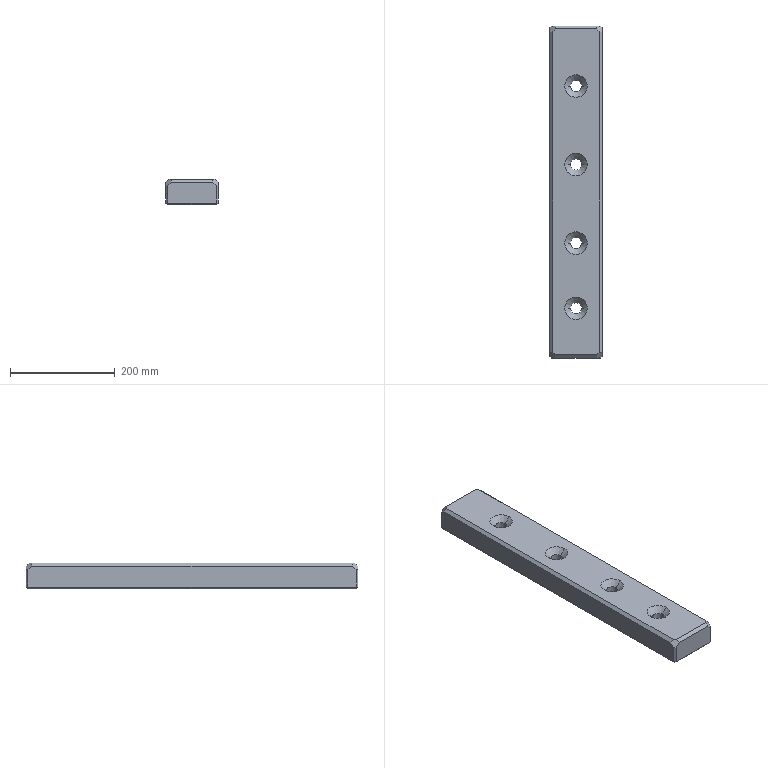Part | Creo | 1 solid | 50 faces | box 100 x 635 x 49.3 mm | volume 3002478 mm3 | plane 26 | cone 16 | cylinder 8 | commonest cylinder face diameters 21.5 x8
STEP:
#1=CARTESIAN_POINT('',(0.,0.,0.));
#2=DIRECTION('',(0.,0.,1.));
#3=DIRECTION('',(1.,0.,0.));
#4=AXIS2_PLACEMENT_3D('',#1,#2,#3);
#5=CARTESIAN_POINT('',(473.372,294.801,305.059));
#6=VERTEX_POINT('',#5);
#7=CARTESIAN_POINT('',(473.372,-319.056,305.059));
#8=VERTEX_POINT('',#7);
#9=CARTESIAN_POINT('',(473.372,294.801,305.059));
#10=DIRECTION('',(0.,-1.,0.));
#11=VECTOR('',#10,613.858);
#12=LINE('',#9,#11);
#13=EDGE_CURVE('',#6,#8,#12,.T.);
#14=ORIENTED_EDGE('',*,*,#13,.T.);
#15=CARTESIAN_POINT('',(468.53,-323.899,305.059));
#16=VERTEX_POINT('',#15);
#17=CARTESIAN_POINT('',(473.372,-319.056,305.059));
#18=DIRECTION('',(-0.7071,-0.7071,0.));
#19=VECTOR('',#18,6.848);
#20=LINE('',#17,#19);
#21=EDGE_CURVE('',#8,#16,#20,.T.);
#22=ORIENTED_EDGE('',*,*,#21,.T.);
#23=CARTESIAN_POINT('',(389.672,-323.899,305.059));
#24=VERTEX_POINT('',#23);
#25=CARTESIAN_POINT('',(468.53,-323.899,305.059));
#26=DIRECTION('',(-1.,0.,0.));
#27=VECTOR('',#26,78.858);
#28=LINE('',#25,#27);
#29=EDGE_CURVE('',#16,#24,#28,.T.);
#30=ORIENTED_EDGE('',*,*,#29,.T.);
#31=CARTESIAN_POINT('',(384.83,-319.056,305.059));
#32=VERTEX_POINT('',#31);
#33=CARTESIAN_POINT('',(389.672,-323.899,305.059));
#34=DIRECTION('',(-0.7071,0.7071,0.));
#35=VECTOR('',#34,6.848);
#36=LINE('',#33,#35);
#37=EDGE_CURVE('',#24,#32,#36,.T.);
#38=ORIENTED_EDGE('',*,*,#37,.T.);
#39=CARTESIAN_POINT('',(384.83,294.801,305.059));
#40=VERTEX_POINT('',#39);
#41=CARTESIAN_POINT('',(384.83,-319.056,305.059));
#42=DIRECTION('',(0.,1.,0.));
#43=VECTOR('',#42,613.858);
#44=LINE('',#41,#43);
#45=EDGE_CURVE('',#32,#40,#44,.T.);
#46=ORIENTED_EDGE('',*,*,#45,.T.);
#47=CARTESIAN_POINT('',(389.672,299.644,305.059));
#48=VERTEX_POINT('',#47);
#49=CARTESIAN_POINT('',(389.672,299.644,305.059));
#50=DIRECTION('',(-0.7071,-0.7071,0.));
#51=VECTOR('',#50,6.848);
#52=LINE('',#49,#51);
#53=EDGE_CURVE('',#48,#40,#52,.T.);
#54=ORIENTED_EDGE('',*,*,#53,.F.);
#55=CARTESIAN_POINT('',(468.53,299.644,305.059));
#56=VERTEX_POINT('',#55);
#57=CARTESIAN_POINT('',(389.672,299.644,305.059));
#58=DIRECTION('',(1.,0.,0.));
#59=VECTOR('',#58,78.858);
#60=LINE('',#57,#59);
#61=EDGE_CURVE('',#48,#56,#60,.T.);
#62=ORIENTED_EDGE('',*,*,#61,.T.);
#63=CARTESIAN_POINT('',(468.53,299.644,305.059));
#64=DIRECTION('',(0.7071,-0.7071,0.));
#65=VECTOR('',#64,6.848);
#66=LINE('',#63,#65);
#67=EDGE_CURVE('',#56,#6,#66,.T.);
#68=ORIENTED_EDGE('',*,*,#67,.T.);
#69=EDGE_LOOP('',(#14,#22,#30,#38,#46,#54,#62,#68));
#70=FACE_OUTER_BOUND('',#69,.F.);
#71=CARTESIAN_POINT('',(450.651,-234.627,305.059));
#72=VERTEX_POINT('',#71);
#73=CARTESIAN_POINT('',(407.551,-234.627,305.059));
#74=VERTEX_POINT('',#73);
#75=CARTESIAN_POINT('',(429.101,-234.627,305.059));
#76=DIRECTION('',(0.,0.,-1.));
#77=DIRECTION('',(1.,0.,0.));
#78=AXIS2_PLACEMENT_3D('',#75,#76,#77);
#79=CIRCLE('',#78,21.55);
#80=EDGE_CURVE('',#72,#74,#79,.T.);
#81=ORIENTED_EDGE('',*,*,#80,.F.);
#82=CARTESIAN_POINT('',(429.101,-234.627,305.059));
#83=DIRECTION('',(0.,0.,-1.));
#84=DIRECTION('',(-1.,0.,0.));
#85=AXIS2_PLACEMENT_3D('',#82,#83,#84);
#86=CIRCLE('',#85,21.55);
#87=EDGE_CURVE('',#74,#72,#86,.T.);
#88=ORIENTED_EDGE('',*,*,#87,.F.);
#89=EDGE_LOOP('',(#81,#88));
#90=FACE_BOUND('',#89,.F.);
#91=CARTESIAN_POINT('',(450.651,-110.,305.059));
#92=VERTEX_POINT('',#91);
#93=CARTESIAN_POINT('',(407.551,-110.,305.059));
#94=VERTEX_POINT('',#93);
#95=CARTESIAN_POINT('',(429.101,-110.,305.059));
#96=DIRECTION('',(0.,0.,-1.));
#97=DIRECTION('',(1.,0.,0.));
#98=AXIS2_PLACEMENT_3D('',#95,#96,#97);
#99=CIRCLE('',#98,21.55);
#100=EDGE_CURVE('',#92,#94,#99,.T.);
#101=ORIENTED_EDGE('',*,*,#100,.F.);
#102=CARTESIAN_POINT('',(429.101,-110.,305.059));
#103=DIRECTION('',(0.,0.,-1.));
#104=DIRECTION('',(-1.,0.,0.));
#105=AXIS2_PLACEMENT_3D('',#102,#103,#104);
#106=CIRCLE('',#105,21.55);
#107=EDGE_CURVE('',#94,#92,#106,.T.);
#108=ORIENTED_EDGE('',*,*,#107,.F.);
#109=EDGE_LOOP('',(#101,#108));
#110=FACE_BOUND('',#109,.F.);
#111=CARTESIAN_POINT('',(450.651,40.373,305.059));
#112=VERTEX_POINT('',#111);
#113=CARTESIAN_POINT('',(407.551,40.373,305.059));
#114=VERTEX_POINT('',#113);
#115=CARTESIAN_POINT('',(429.101,40.373,305.059));
#116=DIRECTION('',(0.,0.,-1.));
#117=DIRECTION('',(1.,0.,0.));
#118=AXIS2_PLACEMENT_3D('',#115,#116,#117);
#119=CIRCLE('',#118,21.55);
#120=EDGE_CURVE('',#112,#114,#119,.T.);
#121=ORIENTED_EDGE('',*,*,#120,.F.);
#122=CARTESIAN_POINT('',(429.101,40.373,305.059));
#123=DIRECTION('',(0.,0.,-1.));
#124=DIRECTION('',(-1.,0.,0.));
#125=AXIS2_PLACEMENT_3D('',#122,#123,#124);
#126=CIRCLE('',#125,21.55);
#127=EDGE_CURVE('',#114,#112,#126,.T.);
#128=ORIENTED_EDGE('',*,*,#127,.F.);
#129=EDGE_LOOP('',(#121,#128));
#130=FACE_BOUND('',#129,.F.);
#131=CARTESIAN_POINT('',(450.651,190.373,305.059));
#132=VERTEX_POINT('',#131);
#133=CARTESIAN_POINT('',(407.551,190.373,305.059));
#134=VERTEX_POINT('',#133);
#135=CARTESIAN_POINT('',(429.101,190.373,305.059));
#136=DIRECTION('',(0.,0.,-1.));
#137=DIRECTION('',(1.,0.,0.));
#138=AXIS2_PLACEMENT_3D('',#135,#136,#137);
#139=CIRCLE('',#138,21.55);
#140=EDGE_CURVE('',#132,#134,#139,.T.);
#141=ORIENTED_EDGE('',*,*,#140,.F.);
#142=CARTESIAN_POINT('',(429.101,190.373,305.059));
#143=DIRECTION('',(0.,0.,-1.));
#144=DIRECTION('',(-1.,0.,0.));
#145=AXIS2_PLACEMENT_3D('',#142,#143,#144);
#146=CIRCLE('',#145,21.55);
#147=EDGE_CURVE('',#134,#132,#146,.T.);
#148=ORIENTED_EDGE('',*,*,#147,.F.);
#149=EDGE_LOOP('',(#141,#148));
#150=FACE_BOUND('',#149,.F.);
#151=CARTESIAN_POINT('',(479.101,305.373,305.059));
#152=DIRECTION('',(0.,0.,1.));
#153=DIRECTION('',(1.,0.,0.));
#154=AXIS2_PLACEMENT_3D('',#151,#152,#153);
#155=PLANE('',#154);
#156=ADVANCED_FACE('',(#70,#90,#110,#130,#150),#155,.T.);
#157=CARTESIAN_POINT('',(479.101,294.801,299.33));
#158=VERTEX_POINT('',#157);
#159=CARTESIAN_POINT('',(473.372,294.801,305.059));
#160=DIRECTION('',(0.7071,0.,-0.7071));
#161=VECTOR('',#160,8.102);
#162=LINE('',#159,#161);
#163=EDGE_CURVE('',#6,#158,#162,.T.);
#164=ORIENTED_EDGE('',*,*,#163,.T.);
#165=CARTESIAN_POINT('',(479.101,-319.056,299.33));
#166=VERTEX_POINT('',#165);
#167=CARTESIAN_POINT('',(479.101,-319.056,299.33));
#168=DIRECTION('',(0.,1.,0.));
#169=VECTOR('',#168,613.858);
#170=LINE('',#167,#169);
#171=EDGE_CURVE('',#166,#158,#170,.T.);
#172=ORIENTED_EDGE('',*,*,#171,.F.);
#173=CARTESIAN_POINT('',(473.372,-319.056,305.059));
#174=DIRECTION('',(0.7071,0.,-0.7071));
#175=VECTOR('',#174,8.102);
#176=LINE('',#173,#175);
#177=EDGE_CURVE('',#8,#166,#176,.T.);
#178=ORIENTED_EDGE('',*,*,#177,.F.);
#179=ORIENTED_EDGE('',*,*,#13,.F.);
#180=EDGE_LOOP('',(#164,#172,#178,#179));
#181=FACE_OUTER_BOUND('',#180,.F.);
#182=CARTESIAN_POINT('',(482.636,305.373,295.794));
#183=DIRECTION('',(-0.7071,0.,-0.7071));
#184=DIRECTION('',(-0.7071,0.,0.7071));
#185=AXIS2_PLACEMENT_3D('',#182,#183,#184);
#186=PLANE('',#185);
#187=ADVANCED_FACE('',(#181),#186,.F.);
#188=ORIENTED_EDGE('',*,*,#67,.F.);
#189=CARTESIAN_POINT('',(468.53,305.373,299.33));
#190=VERTEX_POINT('',#189);
#191=CARTESIAN_POINT('',(468.53,305.373,299.33));
#192=DIRECTION('',(0.,-0.7071,0.7071));
#193=VECTOR('',#192,8.102);
#194=LINE('',#191,#193);
#195=EDGE_CURVE('',#190,#56,#194,.T.);
#196=ORIENTED_EDGE('',*,*,#195,.F.);
#197=CARTESIAN_POINT('',(475.601,305.373,292.259));
#198=VERTEX_POINT('',#197);
#199=CARTESIAN_POINT('',(468.53,305.373,299.33));
#200=DIRECTION('',(0.7071,0.,-0.7071));
#201=VECTOR('',#200,10.);
#202=LINE('',#199,#201);
#203=EDGE_CURVE('',#190,#198,#202,.T.);
#204=ORIENTED_EDGE('',*,*,#203,.T.);
#205=CARTESIAN_POINT('',(479.101,301.873,292.259));
#206=VERTEX_POINT('',#205);
#207=CARTESIAN_POINT('',(479.101,301.873,292.259));
#208=DIRECTION('',(-0.7071,0.7071,0.));
#209=VECTOR('',#208,4.95);
#210=LINE('',#207,#209);
#211=EDGE_CURVE('',#206,#198,#210,.T.);
#212=ORIENTED_EDGE('',*,*,#211,.F.);
#213=CARTESIAN_POINT('',(479.101,294.801,299.33));
#214=DIRECTION('',(0.,0.7071,-0.7071));
#215=VECTOR('',#214,10.);
#216=LINE('',#213,#215);
#217=EDGE_CURVE('',#158,#206,#216,.T.);
#218=ORIENTED_EDGE('',*,*,#217,.F.);
#219=ORIENTED_EDGE('',*,*,#163,.F.);
#220=EDGE_LOOP('',(#188,#196,#204,#212,#218,#219));
#221=FACE_OUTER_BOUND('',#220,.F.);
#222=CARTESIAN_POINT('',(475.601,301.873,295.759));
#223=DIRECTION('',(0.5774,0.5774,0.5774));
#224=DIRECTION('',(0.7071,0.,-0.7071));
#225=AXIS2_PLACEMENT_3D('',#222,#223,#224);
#226=PLANE('',#225);
#227=ADVANCED_FACE('',(#221),#226,.T.);
#228=ORIENTED_EDGE('',*,*,#61,.F.);
#229=CARTESIAN_POINT('',(389.672,305.373,299.33));
#230=VERTEX_POINT('',#229);
#231=CARTESIAN_POINT('',(389.672,299.644,305.059));
#232=DIRECTION('',(0.,0.7071,-0.7071));
#233=VECTOR('',#232,8.102);
#234=LINE('',#231,#233);
#235=EDGE_CURVE('',#48,#230,#234,.T.);
#236=ORIENTED_EDGE('',*,*,#235,.T.);
#237=CARTESIAN_POINT('',(468.53,305.373,299.33));
#238=DIRECTION('',(-1.,0.,0.));
#239=VECTOR('',#238,78.858);
#240=LINE('',#237,#239);
#241=EDGE_CURVE('',#190,#230,#240,.T.);
#242=ORIENTED_EDGE('',*,*,#241,.F.);
#243=ORIENTED_EDGE('',*,*,#195,.T.);
#244=EDGE_LOOP('',(#228,#236,#242,#243));
#245=FACE_OUTER_BOUND('',#244,.F.);
#246=CARTESIAN_POINT('',(479.101,305.408,299.294));
#247=DIRECTION('',(0.,0.7071,0.7071));
#248=DIRECTION('',(0.,-0.7071,0.7071));
#249=AXIS2_PLACEMENT_3D('',#246,#247,#248);
#250=PLANE('',#249);
#251=ADVANCED_FACE('',(#245),#250,.T.);
#252=CARTESIAN_POINT('',(379.101,294.801,299.33));
#253=VERTEX_POINT('',#252);
#254=CARTESIAN_POINT('',(379.101,294.801,299.33));
#255=DIRECTION('',(0.7071,0.,0.7071));
#256=VECTOR('',#255,8.102);
#257=LINE('',#254,#256);
#258=EDGE_CURVE('',#253,#40,#257,.T.);
#259=ORIENTED_EDGE('',*,*,#258,.F.);
#260=CARTESIAN_POINT('',(379.101,301.873,292.259));
#261=VERTEX_POINT('',#260);
#262=CARTESIAN_POINT('',(379.101,294.801,299.33));
#263=DIRECTION('',(0.,0.7071,-0.7071));
#264=VECTOR('',#263,10.);
#265=LINE('',#262,#264);
#266=EDGE_CURVE('',#253,#261,#265,.T.);
#267=ORIENTED_EDGE('',*,*,#266,.T.);
#268=CARTESIAN_POINT('',(382.601,305.373,292.259));
#269=VERTEX_POINT('',#268);
#270=CARTESIAN_POINT('',(382.601,305.373,292.259));
#271=DIRECTION('',(-0.7071,-0.7071,0.));
#272=VECTOR('',#271,4.95);
#273=LINE('',#270,#272);
#274=EDGE_CURVE('',#269,#261,#273,.T.);
#275=ORIENTED_EDGE('',*,*,#274,.F.);
#276=CARTESIAN_POINT('',(382.601,305.373,292.259));
#277=DIRECTION('',(0.7071,0.,0.7071));
#278=VECTOR('',#277,10.);
#279=LINE('',#276,#278);
#280=EDGE_CURVE('',#269,#230,#279,.T.);
#281=ORIENTED_EDGE('',*,*,#280,.T.);
#282=ORIENTED_EDGE('',*,*,#235,.F.);
#283=ORIENTED_EDGE('',*,*,#53,.T.);
#284=EDGE_LOOP('',(#259,#267,#275,#281,#282,#283));
#285=FACE_OUTER_BOUND('',#284,.F.);
#286=CARTESIAN_POINT('',(379.101,301.873,292.259));
#287=DIRECTION('',(-0.5774,0.5774,0.5774));
#288=DIRECTION('',(0.7071,0.,0.7071));
#289=AXIS2_PLACEMENT_3D('',#286,#287,#288);
#290=PLANE('',#289);
#291=ADVANCED_FACE('',(#285),#290,.T.);
#292=ORIENTED_EDGE('',*,*,#45,.F.);
#293=CARTESIAN_POINT('',(379.101,-319.056,299.33));
#294=VERTEX_POINT('',#293);
#295=CARTESIAN_POINT('',(379.101,-319.056,299.33));
#296=DIRECTION('',(0.7071,0.,0.7071));
#297=VECTOR('',#296,8.102);
#298=LINE('',#295,#297);
#299=EDGE_CURVE('',#294,#32,#298,.T.);
#300=ORIENTED_EDGE('',*,*,#299,.F.);
#301=CARTESIAN_POINT('',(379.101,294.801,299.33));
#302=DIRECTION('',(0.,-1.,0.));
#303=VECTOR('',#302,613.858);
#304=LINE('',#301,#303);
#305=EDGE_CURVE('',#253,#294,#304,.T.);
#306=ORIENTED_EDGE('',*,*,#305,.F.);
#307=ORIENTED_EDGE('',*,*,#258,.T.);
#308=EDGE_LOOP('',(#292,#300,#306,#307));
#309=FACE_OUTER_BOUND('',#308,.F.);
#310=CARTESIAN_POINT('',(379.065,305.373,299.294));
#311=DIRECTION('',(-0.7071,0.,0.7071));
#312=DIRECTION('',(0.7071,0.,0.7071));
#313=AXIS2_PLACEMENT_3D('',#310,#311,#312);
#314=PLANE('',#313);
#315=ADVANCED_FACE('',(#309),#314,.T.);
#316=ORIENTED_EDGE('',*,*,#37,.F.);
#317=CARTESIAN_POINT('',(389.672,-329.627,299.33));
#318=VERTEX_POINT('',#317);
#319=CARTESIAN_POINT('',(389.672,-329.627,299.33));
#320=DIRECTION('',(0.,0.7071,0.7071));
#321=VECTOR('',#320,8.102);
#322=LINE('',#319,#321);
#323=EDGE_CURVE('',#318,#24,#322,.T.);
#324=ORIENTED_EDGE('',*,*,#323,.F.);
#325=CARTESIAN_POINT('',(382.601,-329.627,292.259));
#326=VERTEX_POINT('',#325);
#327=CARTESIAN_POINT('',(389.672,-329.627,299.33));
#328=DIRECTION('',(-0.7071,0.,-0.7071));
#329=VECTOR('',#328,10.);
#330=LINE('',#327,#329);
#331=EDGE_CURVE('',#318,#326,#330,.T.);
#332=ORIENTED_EDGE('',*,*,#331,.T.);
#333=CARTESIAN_POINT('',(379.101,-326.127,292.259));
#334=VERTEX_POINT('',#333);
#335=CARTESIAN_POINT('',(379.101,-326.127,292.259));
#336=DIRECTION('',(0.7071,-0.7071,0.));
#337=VECTOR('',#336,4.95);
#338=LINE('',#335,#337);
#339=EDGE_CURVE('',#334,#326,#338,.T.);
#340=ORIENTED_EDGE('',*,*,#339,.F.);
#341=CARTESIAN_POINT('',(379.101,-319.056,299.33));
#342=DIRECTION('',(0.,-0.7071,-0.7071));
#343=VECTOR('',#342,10.);
#344=LINE('',#341,#343);
#345=EDGE_CURVE('',#294,#334,#344,.T.);
#346=ORIENTED_EDGE('',*,*,#345,.F.);
#347=ORIENTED_EDGE('',*,*,#299,.T.);
#348=EDGE_LOOP('',(#316,#324,#332,#340,#346,#347));
#349=FACE_OUTER_BOUND('',#348,.F.);
#350=CARTESIAN_POINT('',(379.101,-326.127,292.259));
#351=DIRECTION('',(-0.5774,-0.5774,0.5774));
#352=DIRECTION('',(0.7071,0.,0.7071));
#353=AXIS2_PLACEMENT_3D('',#350,#351,#352);
#354=PLANE('',#353);
#355=ADVANCED_FACE('',(#349),#354,.T.);
#356=CARTESIAN_POINT('',(468.53,-329.627,299.33));
#357=VERTEX_POINT('',#356);
#358=CARTESIAN_POINT('',(468.53,-323.899,305.059));
#359=DIRECTION('',(0.,-0.7071,-0.7071));
#360=VECTOR('',#359,8.102);
#361=LINE('',#358,#360);
#362=EDGE_CURVE('',#16,#357,#361,.T.);
#363=ORIENTED_EDGE('',*,*,#362,.T.);
#364=CARTESIAN_POINT('',(389.672,-329.627,299.33));
#365=DIRECTION('',(1.,0.,0.));
#366=VECTOR('',#365,78.858);
#367=LINE('',#364,#366);
#368=EDGE_CURVE('',#318,#357,#367,.T.);
#369=ORIENTED_EDGE('',*,*,#368,.F.);
#370=ORIENTED_EDGE('',*,*,#323,.T.);
#371=ORIENTED_EDGE('',*,*,#29,.F.);
#372=EDGE_LOOP('',(#363,#369,#370,#371));
#373=FACE_OUTER_BOUND('',#372,.F.);
#374=CARTESIAN_POINT('',(479.101,-333.163,295.794));
#375=DIRECTION('',(0.,0.7071,-0.7071));
#376=DIRECTION('',(0.,0.7071,0.7071));
#377=AXIS2_PLACEMENT_3D('',#374,#375,#376);
#378=PLANE('',#377);
#379=ADVANCED_FACE('',(#373),#378,.F.);
#380=ORIENTED_EDGE('',*,*,#21,.F.);
#381=ORIENTED_EDGE('',*,*,#177,.T.);
#382=CARTESIAN_POINT('',(479.101,-326.127,292.259));
#383=VERTEX_POINT('',#382);
#384=CARTESIAN_POINT('',(479.101,-319.056,299.33));
#385=DIRECTION('',(0.,-0.7071,-0.7071));
#386=VECTOR('',#385,10.);
#387=LINE('',#384,#386);
#388=EDGE_CURVE('',#166,#383,#387,.T.);
#389=ORIENTED_EDGE('',*,*,#388,.T.);
#390=CARTESIAN_POINT('',(475.601,-329.627,292.259));
#391=VERTEX_POINT('',#390);
#392=CARTESIAN_POINT('',(475.601,-329.627,292.259));
#393=DIRECTION('',(0.7071,0.7071,0.));
#394=VECTOR('',#393,4.95);
#395=LINE('',#392,#394);
#396=EDGE_CURVE('',#391,#383,#395,.T.);
#397=ORIENTED_EDGE('',*,*,#396,.F.);
#398=CARTESIAN_POINT('',(475.601,-329.627,292.259));
#399=DIRECTION('',(-0.7071,0.,0.7071));
#400=VECTOR('',#399,10.);
#401=LINE('',#398,#400);
#402=EDGE_CURVE('',#391,#357,#401,.T.);
#403=ORIENTED_EDGE('',*,*,#402,.T.);
#404=ORIENTED_EDGE('',*,*,#362,.F.);
#405=EDGE_LOOP('',(#380,#381,#389,#397,#403,#404));
#406=FACE_OUTER_BOUND('',#405,.F.);
#407=CARTESIAN_POINT('',(475.601,-329.627,292.259));
#408=DIRECTION('',(0.5774,-0.5774,0.5774));
#409=DIRECTION('',(0.7071,0.,-0.7071));
#410=AXIS2_PLACEMENT_3D('',#407,#408,#409);
#411=PLANE('',#410);
#412=ADVANCED_FACE('',(#406),#411,.T.);
#413=CARTESIAN_POINT('',(479.101,-326.127,259.259));
#414=VERTEX_POINT('',#413);
#415=CARTESIAN_POINT('',(479.101,-326.127,259.259));
#416=DIRECTION('',(0.,0.,1.));
#417=VECTOR('',#416,33.);
#418=LINE('',#415,#417);
#419=EDGE_CURVE('',#414,#383,#418,.T.);
#420=ORIENTED_EDGE('',*,*,#419,.T.);
#421=ORIENTED_EDGE('',*,*,#388,.F.);
#422=ORIENTED_EDGE('',*,*,#171,.T.);
#423=ORIENTED_EDGE('',*,*,#217,.T.);
#424=CARTESIAN_POINT('',(479.101,301.873,259.259));
#425=VERTEX_POINT('',#424);
#426=CARTESIAN_POINT('',(479.101,301.873,292.259));
#427=DIRECTION('',(0.,0.,-1.));
#428=VECTOR('',#427,33.);
#429=LINE('',#426,#428);
#430=EDGE_CURVE('',#206,#425,#429,.T.);
#431=ORIENTED_EDGE('',*,*,#430,.T.);
#432=CARTESIAN_POINT('',(479.101,301.873,259.259));
#433=DIRECTION('',(0.,-1.,0.));
#434=VECTOR('',#433,628.);
#435=LINE('',#432,#434);
#436=EDGE_CURVE('',#425,#414,#435,.T.);
#437=ORIENTED_EDGE('',*,*,#436,.T.);
#438=EDGE_LOOP('',(#420,#421,#422,#423,#431,#437));
#439=FACE_OUTER_BOUND('',#438,.F.);
#440=CARTESIAN_POINT('',(479.101,305.373,290.759));
#441=DIRECTION('',(1.,0.,0.));
#442=DIRECTION('',(0.,1.,0.));
#443=AXIS2_PLACEMENT_3D('',#440,#441,#442);
#444=PLANE('',#443);
#445=ADVANCED_FACE('',(#439),#444,.T.);
#446=CARTESIAN_POINT('',(475.601,-329.627,259.259));
#447=VERTEX_POINT('',#446);
#448=CARTESIAN_POINT('',(479.101,-326.127,259.259));
#449=DIRECTION('',(-0.7071,-0.7071,0.));
#450=VECTOR('',#449,4.95);
#451=LINE('',#448,#450);
#452=EDGE_CURVE('',#414,#447,#451,.T.);
#453=ORIENTED_EDGE('',*,*,#452,.T.);
#454=CARTESIAN_POINT('',(475.601,-329.627,292.259));
#455=DIRECTION('',(0.,0.,-1.));
#456=VECTOR('',#455,33.);
#457=LINE('',#454,#456);
#458=EDGE_CURVE('',#391,#447,#457,.T.);
#459=ORIENTED_EDGE('',*,*,#458,.F.);
#460=ORIENTED_EDGE('',*,*,#396,.T.);
#461=ORIENTED_EDGE('',*,*,#419,.F.);
#462=EDGE_LOOP('',(#453,#459,#460,#461));
#463=FACE_OUTER_BOUND('',#462,.F.);
#464=CARTESIAN_POINT('',(479.101,-326.127,290.759));
#465=DIRECTION('',(-0.7071,0.7071,0.));
#466=DIRECTION('',(-0.7071,-0.7071,0.));
#467=AXIS2_PLACEMENT_3D('',#464,#465,#466);
#468=PLANE('',#467);
#469=ADVANCED_FACE('',(#463),#468,.F.);
#470=CARTESIAN_POINT('',(475.601,-326.127,255.759));
#471=VERTEX_POINT('',#470);
#472=CARTESIAN_POINT('',(479.101,-326.127,259.259));
#473=DIRECTION('',(-0.7071,0.,-0.7071));
#474=VECTOR('',#473,4.95);
#475=LINE('',#472,#474);
#476=EDGE_CURVE('',#414,#471,#475,.T.);
#477=ORIENTED_EDGE('',*,*,#476,.T.);
#478=CARTESIAN_POINT('',(475.601,-329.627,259.259));
#479=DIRECTION('',(0.,0.7071,-0.7071));
#480=VECTOR('',#479,4.95);
#481=LINE('',#478,#480);
#482=EDGE_CURVE('',#447,#471,#481,.T.);
#483=ORIENTED_EDGE('',*,*,#482,.F.);
#484=ORIENTED_EDGE('',*,*,#452,.F.);
#485=EDGE_LOOP('',(#477,#483,#484));
#486=FACE_OUTER_BOUND('',#485,.F.);
#487=CARTESIAN_POINT('',(475.601,-326.127,255.759));
#488=DIRECTION('',(0.5774,-0.5774,-0.5774));
#489=DIRECTION('',(-0.7071,0.,-0.7071));
#490=AXIS2_PLACEMENT_3D('',#487,#488,#489);
#491=PLANE('',#490);
#492=ADVANCED_FACE('',(#486),#491,.T.);
#493=CARTESIAN_POINT('',(475.601,301.873,255.759));
#494=VERTEX_POINT('',#493);
#495=CARTESIAN_POINT('',(479.101,301.873,259.259));
#496=DIRECTION('',(-0.7071,0.,-0.7071));
#497=VECTOR('',#496,4.95);
#498=LINE('',#495,#497);
#499=EDGE_CURVE('',#425,#494,#498,.T.);
#500=ORIENTED_EDGE('',*,*,#499,.T.);
#501=CARTESIAN_POINT('',(475.601,-326.127,255.759));
#502=DIRECTION('',(0.,1.,0.));
#503=VECTOR('',#502,628.);
#504=LINE('',#501,#503);
#505=EDGE_CURVE('',#471,#494,#504,.T.);
#506=ORIENTED_EDGE('',*,*,#505,.F.);
#507=ORIENTED_EDGE('',*,*,#476,.F.);
#508=ORIENTED_EDGE('',*,*,#436,.F.);
#509=EDGE_LOOP('',(#500,#506,#507,#508));
#510=FACE_OUTER_BOUND('',#509,.F.);
#511=CARTESIAN_POINT('',(475.601,305.373,255.759));
#512=DIRECTION('',(0.7071,0.,-0.7071));
#513=DIRECTION('',(-0.7071,0.,-0.7071));
#514=AXIS2_PLACEMENT_3D('',#511,#512,#513);
#515=PLANE('',#514);
#516=ADVANCED_FACE('',(#510),#515,.T.);
#517=CARTESIAN_POINT('',(475.601,305.373,259.259));
#518=VERTEX_POINT('',#517);
#519=CARTESIAN_POINT('',(475.601,301.873,255.759));
#520=DIRECTION('',(0.,0.7071,0.7071));
#521=VECTOR('',#520,4.95);
#522=LINE('',#519,#521);
#523=EDGE_CURVE('',#494,#518,#522,.T.);
#524=ORIENTED_EDGE('',*,*,#523,.F.);
#525=ORIENTED_EDGE('',*,*,#499,.F.);
#526=CARTESIAN_POINT('',(475.601,305.373,259.259));
#527=DIRECTION('',(0.7071,-0.7071,0.));
#528=VECTOR('',#527,4.95);
#529=LINE('',#526,#528);
#530=EDGE_CURVE('',#518,#425,#529,.T.);
#531=ORIENTED_EDGE('',*,*,#530,.F.);
#532=EDGE_LOOP('',(#524,#525,#531));
#533=FACE_OUTER_BOUND('',#532,.F.);
#534=CARTESIAN_POINT('',(475.601,301.873,255.759));
#535=DIRECTION('',(0.5774,0.5774,-0.5774));
#536=DIRECTION('',(-0.7071,0.,-0.7071));
#537=AXIS2_PLACEMENT_3D('',#534,#535,#536);
#538=PLANE('',#537);
#539=ADVANCED_FACE('',(#533),#538,.T.);
#540=ORIENTED_EDGE('',*,*,#523,.T.);
#541=CARTESIAN_POINT('',(382.601,305.373,259.259));
#542=VERTEX_POINT('',#541);
#543=CARTESIAN_POINT('',(382.601,305.373,259.259));
#544=DIRECTION('',(1.,0.,0.));
#545=VECTOR('',#544,93.);
#546=LINE('',#543,#545);
#547=EDGE_CURVE('',#542,#518,#546,.T.);
#548=ORIENTED_EDGE('',*,*,#547,.F.);
#549=CARTESIAN_POINT('',(382.601,301.873,255.759));
#550=VERTEX_POINT('',#549);
#551=CARTESIAN_POINT('',(382.601,305.373,259.259));
#552=DIRECTION('',(0.,-0.7071,-0.7071));
#553=VECTOR('',#552,4.95);
#554=LINE('',#551,#553);
#555=EDGE_CURVE('',#542,#550,#554,.T.);
#556=ORIENTED_EDGE('',*,*,#555,.T.);
#557=CARTESIAN_POINT('',(475.601,301.873,255.759));
#558=DIRECTION('',(-1.,0.,0.));
#559=VECTOR('',#558,93.);
#560=LINE('',#557,#559);
#561=EDGE_CURVE('',#494,#550,#560,.T.);
#562=ORIENTED_EDGE('',*,*,#561,.F.);
#563=EDGE_LOOP('',(#540,#548,#556,#562));
#564=FACE_OUTER_BOUND('',#563,.F.);
#565=CARTESIAN_POINT('',(479.101,305.373,259.259));
#566=DIRECTION('',(0.,-0.7071,0.7071));
#567=DIRECTION('',(0.,-0.7071,-0.7071));
#568=AXIS2_PLACEMENT_3D('',#565,#566,#567);
#569=PLANE('',#568);
#570=ADVANCED_FACE('',(#564),#569,.F.);
#571=ORIENTED_EDGE('',*,*,#241,.T.);
#572=ORIENTED_EDGE('',*,*,#280,.F.);
#573=CARTESIAN_POINT('',(382.601,305.373,292.259));
#574=DIRECTION('',(0.,0.,-1.));
#575=VECTOR('',#574,33.);
#576=LINE('',#573,#575);
#577=EDGE_CURVE('',#269,#542,#576,.T.);
#578=ORIENTED_EDGE('',*,*,#577,.T.);
#579=ORIENTED_EDGE('',*,*,#547,.T.);
#580=CARTESIAN_POINT('',(475.601,305.373,259.259));
#581=DIRECTION('',(0.,0.,1.));
#582=VECTOR('',#581,33.);
#583=LINE('',#580,#582);
#584=EDGE_CURVE('',#518,#198,#583,.T.);
#585=ORIENTED_EDGE('',*,*,#584,.T.);
#586=ORIENTED_EDGE('',*,*,#203,.F.);
#587=EDGE_LOOP('',(#571,#572,#578,#579,#585,#586));
#588=FACE_OUTER_BOUND('',#587,.F.);
#589=CARTESIAN_POINT('',(479.101,305.373,290.759));
#590=DIRECTION('',(0.,-1.,0.));
#591=DIRECTION('',(1.,0.,0.));
#592=AXIS2_PLACEMENT_3D('',#589,#590,#591);
#593=PLANE('',#592);
#594=ADVANCED_FACE('',(#588),#593,.F.);
#595=ORIENTED_EDGE('',*,*,#274,.T.);
#596=CARTESIAN_POINT('',(379.101,301.873,259.259));
#597=VERTEX_POINT('',#596);
#598=CARTESIAN_POINT('',(379.101,301.873,259.259));
#599=DIRECTION('',(0.,0.,1.));
#600=VECTOR('',#599,33.);
#601=LINE('',#598,#600);
#602=EDGE_CURVE('',#597,#261,#601,.T.);
#603=ORIENTED_EDGE('',*,*,#602,.F.);
#604=CARTESIAN_POINT('',(379.101,301.873,259.259));
#605=DIRECTION('',(0.7071,0.7071,0.));
#606=VECTOR('',#605,4.95);
#607=LINE('',#604,#606);
#608=EDGE_CURVE('',#597,#542,#607,.T.);
#609=ORIENTED_EDGE('',*,*,#608,.T.);
#610=ORIENTED_EDGE('',*,*,#577,.F.);
#611=EDGE_LOOP('',(#595,#603,#609,#610));
#612=FACE_OUTER_BOUND('',#611,.F.);
#613=CARTESIAN_POINT('',(379.101,301.873,290.759));
#614=DIRECTION('',(0.7071,-0.7071,0.));
#615=DIRECTION('',(0.7071,0.7071,0.));
#616=AXIS2_PLACEMENT_3D('',#613,#614,#615);
#617=PLANE('',#616);
#618=ADVANCED_FACE('',(#612),#617,.F.);
#619=CARTESIAN_POINT('',(379.101,-326.127,259.259));
#620=VERTEX_POINT('',#619);
#621=CARTESIAN_POINT('',(379.101,-326.127,259.259));
#622=DIRECTION('',(0.,1.,0.));
#623=VECTOR('',#622,628.);
#624=LINE('',#621,#623);
#625=EDGE_CURVE('',#620,#597,#624,.T.);
#626=ORIENTED_EDGE('',*,*,#625,.T.);
#627=ORIENTED_EDGE('',*,*,#602,.T.);
#628=ORIENTED_EDGE('',*,*,#266,.F.);
#629=ORIENTED_EDGE('',*,*,#305,.T.);
#630=ORIENTED_EDGE('',*,*,#345,.T.);
#631=CARTESIAN_POINT('',(379.101,-326.127,292.259));
#632=DIRECTION('',(0.,0.,-1.));
#633=VECTOR('',#632,33.);
#634=LINE('',#631,#633);
#635=EDGE_CURVE('',#334,#620,#634,.T.);
#636=ORIENTED_EDGE('',*,*,#635,.T.);
#637=EDGE_LOOP('',(#626,#627,#628,#629,#630,#636));
#638=FACE_OUTER_BOUND('',#637,.F.);
#639=CARTESIAN_POINT('',(379.101,305.373,290.759));
#640=DIRECTION('',(1.,0.,0.));
#641=DIRECTION('',(0.,1.,0.));
#642=AXIS2_PLACEMENT_3D('',#639,#640,#641);
#643=PLANE('',#642);
#644=ADVANCED_FACE('',(#638),#643,.F.);
#645=CARTESIAN_POINT('',(382.601,301.873,255.759));
#646=DIRECTION('',(-0.7071,0.,0.7071));
#647=VECTOR('',#646,4.95);
#648=LINE('',#645,#647);
#649=EDGE_CURVE('',#550,#597,#648,.T.);
#650=ORIENTED_EDGE('',*,*,#649,.T.);
#651=ORIENTED_EDGE('',*,*,#625,.F.);
#652=CARTESIAN_POINT('',(382.601,-326.127,255.759));
#653=VERTEX_POINT('',#652);
#654=CARTESIAN_POINT('',(382.601,-326.127,255.759));
#655=DIRECTION('',(-0.7071,0.,0.7071));
#656=VECTOR('',#655,4.95);
#657=LINE('',#654,#656);
#658=EDGE_CURVE('',#653,#620,#657,.T.);
#659=ORIENTED_EDGE('',*,*,#658,.F.);
#660=CARTESIAN_POINT('',(382.601,301.873,255.759));
#661=DIRECTION('',(0.,-1.,0.));
#662=VECTOR('',#661,628.);
#663=LINE('',#660,#662);
#664=EDGE_CURVE('',#550,#653,#663,.T.);
#665=ORIENTED_EDGE('',*,*,#664,.F.);
#666=EDGE_LOOP('',(#650,#651,#659,#665));
#667=FACE_OUTER_BOUND('',#666,.F.);
#668=CARTESIAN_POINT('',(379.101,305.373,259.259));
#669=DIRECTION('',(0.7071,0.,0.7071));
#670=DIRECTION('',(0.7071,0.,-0.7071));
#671=AXIS2_PLACEMENT_3D('',#668,#669,#670);
#672=PLANE('',#671);
#673=ADVANCED_FACE('',(#667),#672,.F.);
#674=ORIENTED_EDGE('',*,*,#608,.F.);
#675=ORIENTED_EDGE('',*,*,#649,.F.);
#676=ORIENTED_EDGE('',*,*,#555,.F.);
#677=EDGE_LOOP('',(#674,#675,#676));
#678=FACE_OUTER_BOUND('',#677,.F.);
#679=CARTESIAN_POINT('',(382.601,305.373,259.259));
#680=DIRECTION('',(-0.5774,0.5774,-0.5774));
#681=DIRECTION('',(-0.7071,0.,0.7071));
#682=AXIS2_PLACEMENT_3D('',#679,#680,#681);
#683=PLANE('',#682);
#684=ADVANCED_FACE('',(#678),#683,.T.);
#685=ORIENTED_EDGE('',*,*,#658,.T.);
#686=CARTESIAN_POINT('',(382.601,-329.627,259.259));
#687=VERTEX_POINT('',#686);
#688=CARTESIAN_POINT('',(382.601,-329.627,259.259));
#689=DIRECTION('',(-0.7071,0.7071,0.));
#690=VECTOR('',#689,4.95);
#691=LINE('',#688,#690);
#692=EDGE_CURVE('',#687,#620,#691,.T.);
#693=ORIENTED_EDGE('',*,*,#692,.F.);
#694=CARTESIAN_POINT('',(382.601,-326.127,255.759));
#695=DIRECTION('',(0.,-0.7071,0.7071));
#696=VECTOR('',#695,4.95);
#697=LINE('',#694,#696);
#698=EDGE_CURVE('',#653,#687,#697,.T.);
#699=ORIENTED_EDGE('',*,*,#698,.F.);
#700=EDGE_LOOP('',(#685,#693,#699));
#701=FACE_OUTER_BOUND('',#700,.F.);
#702=CARTESIAN_POINT('',(382.601,-329.627,259.259));
#703=DIRECTION('',(-0.5774,-0.5774,-0.5774));
#704=DIRECTION('',(-0.7071,0.,0.7071));
#705=AXIS2_PLACEMENT_3D('',#702,#703,#704);
#706=PLANE('',#705);
#707=ADVANCED_FACE('',(#701),#706,.T.);
#708=ORIENTED_EDGE('',*,*,#339,.T.);
#709=CARTESIAN_POINT('',(382.601,-329.627,259.259));
#710=DIRECTION('',(0.,0.,1.));
#711=VECTOR('',#710,33.);
#712=LINE('',#709,#711);
#713=EDGE_CURVE('',#687,#326,#712,.T.);
#714=ORIENTED_EDGE('',*,*,#713,.F.);
#715=ORIENTED_EDGE('',*,*,#692,.T.);
#716=ORIENTED_EDGE('',*,*,#635,.F.);
#717=EDGE_LOOP('',(#708,#714,#715,#716));
#718=FACE_OUTER_BOUND('',#717,.F.);
#719=CARTESIAN_POINT('',(382.601,-329.627,290.759));
#720=DIRECTION('',(-0.7071,-0.7071,0.));
#721=DIRECTION('',(0.7071,-0.7071,0.));
#722=AXIS2_PLACEMENT_3D('',#719,#720,#721);
#723=PLANE('',#722);
#724=ADVANCED_FACE('',(#718),#723,.T.);
#725=ORIENTED_EDGE('',*,*,#368,.T.);
#726=ORIENTED_EDGE('',*,*,#402,.F.);
#727=ORIENTED_EDGE('',*,*,#458,.T.);
#728=CARTESIAN_POINT('',(475.601,-329.627,259.259));
#729=DIRECTION('',(-1.,0.,0.));
#730=VECTOR('',#729,93.);
#731=LINE('',#728,#730);
#732=EDGE_CURVE('',#447,#687,#731,.T.);
#733=ORIENTED_EDGE('',*,*,#732,.T.);
#734=ORIENTED_EDGE('',*,*,#713,.T.);
#735=ORIENTED_EDGE('',*,*,#331,.F.);
#736=EDGE_LOOP('',(#725,#726,#727,#733,#734,#735));
#737=FACE_OUTER_BOUND('',#736,.F.);
#738=CARTESIAN_POINT('',(479.101,-329.627,290.759));
#739=DIRECTION('',(0.,-1.,0.));
#740=DIRECTION('',(1.,0.,0.));
#741=AXIS2_PLACEMENT_3D('',#738,#739,#740);
#742=PLANE('',#741);
#743=ADVANCED_FACE('',(#737),#742,.T.);
#744=ORIENTED_EDGE('',*,*,#482,.T.);
#745=CARTESIAN_POINT('',(382.601,-326.127,255.759));
#746=DIRECTION('',(1.,0.,0.));
#747=VECTOR('',#746,93.);
#748=LINE('',#745,#747);
#749=EDGE_CURVE('',#653,#471,#748,.T.);
#750=ORIENTED_EDGE('',*,*,#749,.F.);
#751=ORIENTED_EDGE('',*,*,#698,.T.);
#752=ORIENTED_EDGE('',*,*,#732,.F.);
#753=EDGE_LOOP('',(#744,#750,#751,#752));
#754=FACE_OUTER_BOUND('',#753,.F.);
#755=CARTESIAN_POINT('',(479.101,-326.127,255.759));
#756=DIRECTION('',(0.,-0.7071,-0.7071));
#757=DIRECTION('',(0.,0.7071,-0.7071));
#758=AXIS2_PLACEMENT_3D('',#755,#756,#757);
#759=PLANE('',#758);
#760=ADVANCED_FACE('',(#754),#759,.T.);
#761=ORIENTED_EDGE('',*,*,#664,.T.);
#762=ORIENTED_EDGE('',*,*,#749,.T.);
#763=ORIENTED_EDGE('',*,*,#505,.T.);
#764=ORIENTED_EDGE('',*,*,#561,.T.);
#765=EDGE_LOOP('',(#761,#762,#763,#764));
#766=FACE_OUTER_BOUND('',#765,.F.);
#767=CARTESIAN_POINT('',(441.351,40.373,255.759));
#768=VERTEX_POINT('',#767);
#769=CARTESIAN_POINT('',(416.851,40.373,255.759));
#770=VERTEX_POINT('',#769);
#771=CARTESIAN_POINT('',(429.101,40.373,255.759));
#772=DIRECTION('',(0.,0.,1.));
#773=DIRECTION('',(1.,0.,0.));
#774=AXIS2_PLACEMENT_3D('',#771,#772,#773);
#775=CIRCLE('',#774,12.25);
#776=EDGE_CURVE('',#768,#770,#775,.T.);
#777=ORIENTED_EDGE('',*,*,#776,.F.);
#778=CARTESIAN_POINT('',(429.101,40.373,255.759));
#779=DIRECTION('',(0.,0.,1.));
#780=DIRECTION('',(-1.,0.,0.));
#781=AXIS2_PLACEMENT_3D('',#778,#779,#780);
#782=CIRCLE('',#781,12.25);
#783=EDGE_CURVE('',#770,#768,#782,.T.);
#784=ORIENTED_EDGE('',*,*,#783,.F.);
#785=EDGE_LOOP('',(#777,#784));
#786=FACE_BOUND('',#785,.F.);
#787=CARTESIAN_POINT('',(441.351,-110.,255.759));
#788=VERTEX_POINT('',#787);
#789=CARTESIAN_POINT('',(416.851,-110.,255.759));
#790=VERTEX_POINT('',#789);
#791=CARTESIAN_POINT('',(429.101,-110.,255.759));
#792=DIRECTION('',(0.,0.,1.));
#793=DIRECTION('',(1.,0.,0.));
#794=AXIS2_PLACEMENT_3D('',#791,#792,#793);
#795=CIRCLE('',#794,12.25);
#796=EDGE_CURVE('',#788,#790,#795,.T.);
#797=ORIENTED_EDGE('',*,*,#796,.F.);
#798=CARTESIAN_POINT('',(429.101,-110.,255.759));
#799=DIRECTION('',(0.,0.,1.));
#800=DIRECTION('',(-1.,0.,0.));
#801=AXIS2_PLACEMENT_3D('',#798,#799,#800);
#802=CIRCLE('',#801,12.25);
#803=EDGE_CURVE('',#790,#788,#802,.T.);
#804=ORIENTED_EDGE('',*,*,#803,.F.);
#805=EDGE_LOOP('',(#797,#804));
#806=FACE_BOUND('',#805,.F.);
#807=CARTESIAN_POINT('',(441.351,-234.627,255.759));
#808=VERTEX_POINT('',#807);
#809=CARTESIAN_POINT('',(416.851,-234.627,255.759));
#810=VERTEX_POINT('',#809);
#811=CARTESIAN_POINT('',(429.101,-234.627,255.759));
#812=DIRECTION('',(0.,0.,1.));
#813=DIRECTION('',(1.,0.,0.));
#814=AXIS2_PLACEMENT_3D('',#811,#812,#813);
#815=CIRCLE('',#814,12.25);
#816=EDGE_CURVE('',#808,#810,#815,.T.);
#817=ORIENTED_EDGE('',*,*,#816,.F.);
#818=CARTESIAN_POINT('',(429.101,-234.627,255.759));
#819=DIRECTION('',(0.,0.,1.));
#820=DIRECTION('',(-1.,0.,0.));
#821=AXIS2_PLACEMENT_3D('',#818,#819,#820);
#822=CIRCLE('',#821,12.25);
#823=EDGE_CURVE('',#810,#808,#822,.T.);
#824=ORIENTED_EDGE('',*,*,#823,.F.);
#825=EDGE_LOOP('',(#817,#824));
#826=FACE_BOUND('',#825,.F.);
#827=CARTESIAN_POINT('',(441.351,190.373,255.759));
#828=VERTEX_POINT('',#827);
#829=CARTESIAN_POINT('',(416.851,190.373,255.759));
#830=VERTEX_POINT('',#829);
#831=CARTESIAN_POINT('',(429.101,190.373,255.759));
#832=DIRECTION('',(0.,0.,1.));
#833=DIRECTION('',(1.,0.,0.));
#834=AXIS2_PLACEMENT_3D('',#831,#832,#833);
#835=CIRCLE('',#834,12.25);
#836=EDGE_CURVE('',#828,#830,#835,.T.);
#837=ORIENTED_EDGE('',*,*,#836,.F.);
#838=CARTESIAN_POINT('',(429.101,190.373,255.759));
#839=DIRECTION('',(0.,0.,1.));
#840=DIRECTION('',(-1.,0.,0.));
#841=AXIS2_PLACEMENT_3D('',#838,#839,#840);
#842=CIRCLE('',#841,12.25);
#843=EDGE_CURVE('',#830,#828,#842,.T.);
#844=ORIENTED_EDGE('',*,*,#843,.F.);
#845=EDGE_LOOP('',(#837,#844));
#846=FACE_BOUND('',#845,.F.);
#847=CARTESIAN_POINT('',(479.101,305.373,255.759));
#848=DIRECTION('',(0.,0.,1.));
#849=DIRECTION('',(1.,0.,0.));
#850=AXIS2_PLACEMENT_3D('',#847,#848,#849);
#851=PLANE('',#850);
#852=ADVANCED_FACE('',(#766,#786,#806,#826,#846),#851,.F.);
#853=ORIENTED_EDGE('',*,*,#836,.T.);
#854=CARTESIAN_POINT('',(418.351,190.373,257.259));
#855=VERTEX_POINT('',#854);
#856=CARTESIAN_POINT('',(418.351,190.373,257.259));
#857=DIRECTION('',(-0.7071,0.,-0.7071));
#858=VECTOR('',#857,2.121);
#859=LINE('',#856,#858);
#860=EDGE_CURVE('',#855,#830,#859,.T.);
#861=ORIENTED_EDGE('',*,*,#860,.F.);
#862=CARTESIAN_POINT('',(439.851,190.373,257.259));
#863=VERTEX_POINT('',#862);
#864=CARTESIAN_POINT('',(429.101,190.373,257.259));
#865=DIRECTION('',(0.,0.,1.));
#866=DIRECTION('',(1.,0.,0.));
#867=AXIS2_PLACEMENT_3D('',#864,#865,#866);
#868=CIRCLE('',#867,10.75);
#869=EDGE_CURVE('',#863,#855,#868,.T.);
#870=ORIENTED_EDGE('',*,*,#869,.F.);
#871=CARTESIAN_POINT('',(439.851,190.373,257.259));
#872=DIRECTION('',(0.7071,0.,-0.7071));
#873=VECTOR('',#872,2.121);
#874=LINE('',#871,#873);
#875=EDGE_CURVE('',#863,#828,#874,.T.);
#876=ORIENTED_EDGE('',*,*,#875,.T.);
#877=EDGE_LOOP('',(#853,#861,#870,#876));
#878=FACE_OUTER_BOUND('',#877,.F.);
#879=CARTESIAN_POINT('',(429.101,190.373,256.509));
#880=DIRECTION('',(0.,0.,-1.));
#881=DIRECTION('',(-1.,0.,0.));
#882=AXIS2_PLACEMENT_3D('',#879,#880,#881);
#883=CONICAL_SURFACE('',#882,11.5,45.);
#884=ADVANCED_FACE('',(#878),#883,.F.);
#885=ORIENTED_EDGE('',*,*,#843,.T.);
#886=ORIENTED_EDGE('',*,*,#875,.F.);
#887=CARTESIAN_POINT('',(429.101,190.373,257.259));
#888=DIRECTION('',(0.,0.,1.));
#889=DIRECTION('',(-1.,0.,0.));
#890=AXIS2_PLACEMENT_3D('',#887,#888,#889);
#891=CIRCLE('',#890,10.75);
#892=EDGE_CURVE('',#855,#863,#891,.T.);
#893=ORIENTED_EDGE('',*,*,#892,.F.);
#894=ORIENTED_EDGE('',*,*,#860,.T.);
#895=EDGE_LOOP('',(#885,#886,#893,#894));
#896=FACE_OUTER_BOUND('',#895,.F.);
#897=CARTESIAN_POINT('',(429.101,190.373,256.509));
#898=DIRECTION('',(0.,0.,-1.));
#899=DIRECTION('',(-1.,0.,0.));
#900=AXIS2_PLACEMENT_3D('',#897,#898,#899);
#901=CONICAL_SURFACE('',#900,11.5,45.);
#902=ADVANCED_FACE('',(#896),#901,.F.);
#903=CARTESIAN_POINT('',(439.851,190.373,294.259));
#904=VERTEX_POINT('',#903);
#905=CARTESIAN_POINT('',(418.351,190.373,294.259));
#906=VERTEX_POINT('',#905);
#907=CARTESIAN_POINT('',(429.101,190.373,294.259));
#908=DIRECTION('',(0.,0.,-1.));
#909=DIRECTION('',(1.,0.,0.));
#910=AXIS2_PLACEMENT_3D('',#907,#908,#909);
#911=CIRCLE('',#910,10.75);
#912=EDGE_CURVE('',#904,#906,#911,.T.);
#913=ORIENTED_EDGE('',*,*,#912,.T.);
#914=CARTESIAN_POINT('',(418.351,190.373,294.259));
#915=DIRECTION('',(0.,0.,-1.));
#916=VECTOR('',#915,37.);
#917=LINE('',#914,#916);
#918=EDGE_CURVE('',#906,#855,#917,.T.);
#919=ORIENTED_EDGE('',*,*,#918,.T.);
#920=ORIENTED_EDGE('',*,*,#892,.T.);
#921=CARTESIAN_POINT('',(439.851,190.373,294.259));
#922=DIRECTION('',(0.,0.,-1.));
#923=VECTOR('',#922,37.);
#924=LINE('',#921,#923);
#925=EDGE_CURVE('',#904,#863,#924,.T.);
#926=ORIENTED_EDGE('',*,*,#925,.F.);
#927=EDGE_LOOP('',(#913,#919,#920,#926));
#928=FACE_OUTER_BOUND('',#927,.F.);
#929=CARTESIAN_POINT('',(429.101,190.373,344.759));
#930=DIRECTION('',(0.,0.,-1.));
#931=DIRECTION('',(-1.,0.,0.));
#932=AXIS2_PLACEMENT_3D('',#929,#930,#931);
#933=CYLINDRICAL_SURFACE('',#932,10.75);
#934=ADVANCED_FACE('',(#928),#933,.F.);
#935=ORIENTED_EDGE('',*,*,#140,.T.);
#936=CARTESIAN_POINT('',(418.351,190.373,294.259));
#937=DIRECTION('',(-0.7071,0.,0.7071));
#938=VECTOR('',#937,15.274);
#939=LINE('',#936,#938);
#940=EDGE_CURVE('',#906,#134,#939,.T.);
#941=ORIENTED_EDGE('',*,*,#940,.F.);
#942=ORIENTED_EDGE('',*,*,#912,.F.);
#943=CARTESIAN_POINT('',(439.851,190.373,294.259));
#944=DIRECTION('',(0.7071,0.,0.7071));
#945=VECTOR('',#944,15.274);
#946=LINE('',#943,#945);
#947=EDGE_CURVE('',#904,#132,#946,.T.);
#948=ORIENTED_EDGE('',*,*,#947,.T.);
#949=EDGE_LOOP('',(#935,#941,#942,#948));
#950=FACE_OUTER_BOUND('',#949,.F.);
#951=CARTESIAN_POINT('',(429.101,190.373,299.659));
#952=DIRECTION('',(0.,0.,1.));
#953=DIRECTION('',(1.,0.,0.));
#954=AXIS2_PLACEMENT_3D('',#951,#952,#953);
#955=CONICAL_SURFACE('',#954,16.15,45.);
#956=ADVANCED_FACE('',(#950),#955,.F.);
#957=ORIENTED_EDGE('',*,*,#147,.T.);
#958=ORIENTED_EDGE('',*,*,#947,.F.);
#959=CARTESIAN_POINT('',(429.101,190.373,294.259));
#960=DIRECTION('',(0.,0.,-1.));
#961=DIRECTION('',(-1.,0.,0.));
#962=AXIS2_PLACEMENT_3D('',#959,#960,#961);
#963=CIRCLE('',#962,10.75);
#964=EDGE_CURVE('',#906,#904,#963,.T.);
#965=ORIENTED_EDGE('',*,*,#964,.F.);
#966=ORIENTED_EDGE('',*,*,#940,.T.);
#967=EDGE_LOOP('',(#957,#958,#965,#966));
#968=FACE_OUTER_BOUND('',#967,.F.);
#969=CARTESIAN_POINT('',(429.101,190.373,299.659));
#970=DIRECTION('',(0.,0.,1.));
#971=DIRECTION('',(1.,0.,0.));
#972=AXIS2_PLACEMENT_3D('',#969,#970,#971);
#973=CONICAL_SURFACE('',#972,16.15,45.);
#974=ADVANCED_FACE('',(#968),#973,.F.);
#975=ORIENTED_EDGE('',*,*,#964,.T.);
#976=ORIENTED_EDGE('',*,*,#925,.T.);
#977=ORIENTED_EDGE('',*,*,#869,.T.);
#978=ORIENTED_EDGE('',*,*,#918,.F.);
#979=EDGE_LOOP('',(#975,#976,#977,#978));
#980=FACE_OUTER_BOUND('',#979,.F.);
#981=CARTESIAN_POINT('',(429.101,190.373,344.759));
#982=DIRECTION('',(0.,0.,-1.));
#983=DIRECTION('',(-1.,0.,0.));
#984=AXIS2_PLACEMENT_3D('',#981,#982,#983);
#985=CYLINDRICAL_SURFACE('',#984,10.75);
#986=ADVANCED_FACE('',(#980),#985,.F.);
#987=ORIENTED_EDGE('',*,*,#776,.T.);
#988=CARTESIAN_POINT('',(418.351,40.373,257.259));
#989=VERTEX_POINT('',#988);
#990=CARTESIAN_POINT('',(418.351,40.373,257.259));
#991=DIRECTION('',(-0.7071,0.,-0.7071));
#992=VECTOR('',#991,2.121);
#993=LINE('',#990,#992);
#994=EDGE_CURVE('',#989,#770,#993,.T.);
#995=ORIENTED_EDGE('',*,*,#994,.F.);
#996=CARTESIAN_POINT('',(439.851,40.373,257.259));
#997=VERTEX_POINT('',#996);
#998=CARTESIAN_POINT('',(429.101,40.373,257.259));
#999=DIRECTION('',(0.,0.,1.));
#1000=DIRECTION('',(1.,0.,0.));
#1001=AXIS2_PLACEMENT_3D('',#998,#999,#1000);
#1002=CIRCLE('',#1001,10.75);
#1003=EDGE_CURVE('',#997,#989,#1002,.T.);
#1004=ORIENTED_EDGE('',*,*,#1003,.F.);
#1005=CARTESIAN_POINT('',(439.851,40.373,257.259));
#1006=DIRECTION('',(0.7071,0.,-0.7071));
#1007=VECTOR('',#1006,2.121);
#1008=LINE('',#1005,#1007);
#1009=EDGE_CURVE('',#997,#768,#1008,.T.);
#1010=ORIENTED_EDGE('',*,*,#1009,.T.);
#1011=EDGE_LOOP('',(#987,#995,#1004,#1010));
#1012=FACE_OUTER_BOUND('',#1011,.F.);
#1013=CARTESIAN_POINT('',(429.101,40.373,256.509));
#1014=DIRECTION('',(0.,0.,-1.));
#1015=DIRECTION('',(-1.,0.,0.));
#1016=AXIS2_PLACEMENT_3D('',#1013,#1014,#1015);
#1017=CONICAL_SURFACE('',#1016,11.5,45.);
#1018=ADVANCED_FACE('',(#1012),#1017,.F.);
#1019=ORIENTED_EDGE('',*,*,#783,.T.);
#1020=ORIENTED_EDGE('',*,*,#1009,.F.);
#1021=CARTESIAN_POINT('',(429.101,40.373,257.259));
#1022=DIRECTION('',(0.,0.,1.));
#1023=DIRECTION('',(-1.,0.,0.));
#1024=AXIS2_PLACEMENT_3D('',#1021,#1022,#1023);
#1025=CIRCLE('',#1024,10.75);
#1026=EDGE_CURVE('',#989,#997,#1025,.T.);
#1027=ORIENTED_EDGE('',*,*,#1026,.F.);
#1028=ORIENTED_EDGE('',*,*,#994,.T.);
#1029=EDGE_LOOP('',(#1019,#1020,#1027,#1028));
#1030=FACE_OUTER_BOUND('',#1029,.F.);
#1031=CARTESIAN_POINT('',(429.101,40.373,256.509));
#1032=DIRECTION('',(0.,0.,-1.));
#1033=DIRECTION('',(-1.,0.,0.));
#1034=AXIS2_PLACEMENT_3D('',#1031,#1032,#1033);
#1035=CONICAL_SURFACE('',#1034,11.5,45.);
#1036=ADVANCED_FACE('',(#1030),#1035,.F.);
#1037=CARTESIAN_POINT('',(439.851,40.373,294.259));
#1038=VERTEX_POINT('',#1037);
#1039=CARTESIAN_POINT('',(418.351,40.373,294.259));
#1040=VERTEX_POINT('',#1039);
#1041=CARTESIAN_POINT('',(429.101,40.373,294.259));
#1042=DIRECTION('',(0.,0.,-1.));
#1043=DIRECTION('',(1.,0.,0.));
#1044=AXIS2_PLACEMENT_3D('',#1041,#1042,#1043);
#1045=CIRCLE('',#1044,10.75);
#1046=EDGE_CURVE('',#1038,#1040,#1045,.T.);
#1047=ORIENTED_EDGE('',*,*,#1046,.T.);
#1048=CARTESIAN_POINT('',(418.351,40.373,294.259));
#1049=DIRECTION('',(0.,0.,-1.));
#1050=VECTOR('',#1049,37.);
#1051=LINE('',#1048,#1050);
#1052=EDGE_CURVE('',#1040,#989,#1051,.T.);
#1053=ORIENTED_EDGE('',*,*,#1052,.T.);
#1054=ORIENTED_EDGE('',*,*,#1026,.T.);
#1055=CARTESIAN_POINT('',(439.851,40.373,294.259));
#1056=DIRECTION('',(0.,0.,-1.));
#1057=VECTOR('',#1056,37.);
#1058=LINE('',#1055,#1057);
#1059=EDGE_CURVE('',#1038,#997,#1058,.T.);
#1060=ORIENTED_EDGE('',*,*,#1059,.F.);
#1061=EDGE_LOOP('',(#1047,#1053,#1054,#1060));
#1062=FACE_OUTER_BOUND('',#1061,.F.);
#1063=CARTESIAN_POINT('',(429.101,40.373,344.759));
#1064=DIRECTION('',(0.,0.,-1.));
#1065=DIRECTION('',(-1.,0.,0.));
#1066=AXIS2_PLACEMENT_3D('',#1063,#1064,#1065);
#1067=CYLINDRICAL_SURFACE('',#1066,10.75);
#1068=ADVANCED_FACE('',(#1062),#1067,.F.);
#1069=ORIENTED_EDGE('',*,*,#120,.T.);
#1070=CARTESIAN_POINT('',(418.351,40.373,294.259));
#1071=DIRECTION('',(-0.7071,0.,0.7071));
#1072=VECTOR('',#1071,15.274);
#1073=LINE('',#1070,#1072);
#1074=EDGE_CURVE('',#1040,#114,#1073,.T.);
#1075=ORIENTED_EDGE('',*,*,#1074,.F.);
#1076=ORIENTED_EDGE('',*,*,#1046,.F.);
#1077=CARTESIAN_POINT('',(439.851,40.373,294.259));
#1078=DIRECTION('',(0.7071,0.,0.7071));
#1079=VECTOR('',#1078,15.274);
#1080=LINE('',#1077,#1079);
#1081=EDGE_CURVE('',#1038,#112,#1080,.T.);
#1082=ORIENTED_EDGE('',*,*,#1081,.T.);
#1083=EDGE_LOOP('',(#1069,#1075,#1076,#1082));
#1084=FACE_OUTER_BOUND('',#1083,.F.);
#1085=CARTESIAN_POINT('',(429.101,40.373,299.659));
#1086=DIRECTION('',(0.,0.,1.));
#1087=DIRECTION('',(1.,0.,0.));
#1088=AXIS2_PLACEMENT_3D('',#1085,#1086,#1087);
#1089=CONICAL_SURFACE('',#1088,16.15,45.);
#1090=ADVANCED_FACE('',(#1084),#1089,.F.);
#1091=ORIENTED_EDGE('',*,*,#127,.T.);
#1092=ORIENTED_EDGE('',*,*,#1081,.F.);
#1093=CARTESIAN_POINT('',(429.101,40.373,294.259));
#1094=DIRECTION('',(0.,0.,-1.));
#1095=DIRECTION('',(-1.,0.,0.));
#1096=AXIS2_PLACEMENT_3D('',#1093,#1094,#1095);
#1097=CIRCLE('',#1096,10.75);
#1098=EDGE_CURVE('',#1040,#1038,#1097,.T.);
#1099=ORIENTED_EDGE('',*,*,#1098,.F.);
#1100=ORIENTED_EDGE('',*,*,#1074,.T.);
#1101=EDGE_LOOP('',(#1091,#1092,#1099,#1100));
#1102=FACE_OUTER_BOUND('',#1101,.F.);
#1103=CARTESIAN_POINT('',(429.101,40.373,299.659));
#1104=DIRECTION('',(0.,0.,1.));
#1105=DIRECTION('',(1.,0.,0.));
#1106=AXIS2_PLACEMENT_3D('',#1103,#1104,#1105);
#1107=CONICAL_SURFACE('',#1106,16.15,45.);
#1108=ADVANCED_FACE('',(#1102),#1107,.F.);
#1109=ORIENTED_EDGE('',*,*,#1098,.T.);
#1110=ORIENTED_EDGE('',*,*,#1059,.T.);
#1111=ORIENTED_EDGE('',*,*,#1003,.T.);
#1112=ORIENTED_EDGE('',*,*,#1052,.F.);
#1113=EDGE_LOOP('',(#1109,#1110,#1111,#1112));
#1114=FACE_OUTER_BOUND('',#1113,.F.);
#1115=CARTESIAN_POINT('',(429.101,40.373,344.759));
#1116=DIRECTION('',(0.,0.,-1.));
#1117=DIRECTION('',(-1.,0.,0.));
#1118=AXIS2_PLACEMENT_3D('',#1115,#1116,#1117);
#1119=CYLINDRICAL_SURFACE('',#1118,10.75);
#1120=ADVANCED_FACE('',(#1114),#1119,.F.);
#1121=ORIENTED_EDGE('',*,*,#796,.T.);
#1122=CARTESIAN_POINT('',(418.351,-110.,257.259));
#1123=VERTEX_POINT('',#1122);
#1124=CARTESIAN_POINT('',(418.351,-110.,257.259));
#1125=DIRECTION('',(-0.7071,0.,-0.7071));
#1126=VECTOR('',#1125,2.121);
#1127=LINE('',#1124,#1126);
#1128=EDGE_CURVE('',#1123,#790,#1127,.T.);
#1129=ORIENTED_EDGE('',*,*,#1128,.F.);
#1130=CARTESIAN_POINT('',(439.851,-110.,257.259));
#1131=VERTEX_POINT('',#1130);
#1132=CARTESIAN_POINT('',(429.101,-110.,257.259));
#1133=DIRECTION('',(0.,0.,1.));
#1134=DIRECTION('',(1.,0.,0.));
#1135=AXIS2_PLACEMENT_3D('',#1132,#1133,#1134);
#1136=CIRCLE('',#1135,10.75);
#1137=EDGE_CURVE('',#1131,#1123,#1136,.T.);
#1138=ORIENTED_EDGE('',*,*,#1137,.F.);
#1139=CARTESIAN_POINT('',(439.851,-110.,257.259));
#1140=DIRECTION('',(0.7071,0.,-0.7071));
#1141=VECTOR('',#1140,2.121);
#1142=LINE('',#1139,#1141);
#1143=EDGE_CURVE('',#1131,#788,#1142,.T.);
#1144=ORIENTED_EDGE('',*,*,#1143,.T.);
#1145=EDGE_LOOP('',(#1121,#1129,#1138,#1144));
#1146=FACE_OUTER_BOUND('',#1145,.F.);
#1147=CARTESIAN_POINT('',(429.101,-110.,256.509));
#1148=DIRECTION('',(0.,0.,-1.));
#1149=DIRECTION('',(-1.,0.,0.));
#1150=AXIS2_PLACEMENT_3D('',#1147,#1148,#1149);
#1151=CONICAL_SURFACE('',#1150,11.5,45.);
#1152=ADVANCED_FACE('',(#1146),#1151,.F.);
#1153=ORIENTED_EDGE('',*,*,#803,.T.);
#1154=ORIENTED_EDGE('',*,*,#1143,.F.);
#1155=CARTESIAN_POINT('',(429.101,-110.,257.259));
#1156=DIRECTION('',(0.,0.,1.));
#1157=DIRECTION('',(-1.,0.,0.));
#1158=AXIS2_PLACEMENT_3D('',#1155,#1156,#1157);
#1159=CIRCLE('',#1158,10.75);
#1160=EDGE_CURVE('',#1123,#1131,#1159,.T.);
#1161=ORIENTED_EDGE('',*,*,#1160,.F.);
#1162=ORIENTED_EDGE('',*,*,#1128,.T.);
#1163=EDGE_LOOP('',(#1153,#1154,#1161,#1162));
#1164=FACE_OUTER_BOUND('',#1163,.F.);
#1165=CARTESIAN_POINT('',(429.101,-110.,256.509));
#1166=DIRECTION('',(0.,0.,-1.));
#1167=DIRECTION('',(-1.,0.,0.));
#1168=AXIS2_PLACEMENT_3D('',#1165,#1166,#1167);
#1169=CONICAL_SURFACE('',#1168,11.5,45.);
#1170=ADVANCED_FACE('',(#1164),#1169,.F.);
#1171=CARTESIAN_POINT('',(439.851,-110.,294.259));
#1172=VERTEX_POINT('',#1171);
#1173=CARTESIAN_POINT('',(418.351,-110.,294.259));
#1174=VERTEX_POINT('',#1173);
#1175=CARTESIAN_POINT('',(429.101,-110.,294.259));
#1176=DIRECTION('',(0.,0.,-1.));
#1177=DIRECTION('',(1.,0.,0.));
#1178=AXIS2_PLACEMENT_3D('',#1175,#1176,#1177);
#1179=CIRCLE('',#1178,10.75);
#1180=EDGE_CURVE('',#1172,#1174,#1179,.T.);
#1181=ORIENTED_EDGE('',*,*,#1180,.T.);
#1182=CARTESIAN_POINT('',(418.351,-110.,294.259));
#1183=DIRECTION('',(0.,0.,-1.));
#1184=VECTOR('',#1183,37.);
#1185=LINE('',#1182,#1184);
#1186=EDGE_CURVE('',#1174,#1123,#1185,.T.);
#1187=ORIENTED_EDGE('',*,*,#1186,.T.);
#1188=ORIENTED_EDGE('',*,*,#1160,.T.);
#1189=CARTESIAN_POINT('',(439.851,-110.,294.259));
#1190=DIRECTION('',(0.,0.,-1.));
#1191=VECTOR('',#1190,37.);
#1192=LINE('',#1189,#1191);
#1193=EDGE_CURVE('',#1172,#1131,#1192,.T.);
#1194=ORIENTED_EDGE('',*,*,#1193,.F.);
#1195=EDGE_LOOP('',(#1181,#1187,#1188,#1194));
#1196=FACE_OUTER_BOUND('',#1195,.F.);
#1197=CARTESIAN_POINT('',(429.101,-110.,344.759));
#1198=DIRECTION('',(0.,0.,-1.));
#1199=DIRECTION('',(-1.,0.,0.));
#1200=AXIS2_PLACEMENT_3D('',#1197,#1198,#1199);
#1201=CYLINDRICAL_SURFACE('',#1200,10.75);
#1202=ADVANCED_FACE('',(#1196),#1201,.F.);
#1203=ORIENTED_EDGE('',*,*,#100,.T.);
#1204=CARTESIAN_POINT('',(418.351,-110.,294.259));
#1205=DIRECTION('',(-0.7071,0.,0.7071));
#1206=VECTOR('',#1205,15.274);
#1207=LINE('',#1204,#1206);
#1208=EDGE_CURVE('',#1174,#94,#1207,.T.);
#1209=ORIENTED_EDGE('',*,*,#1208,.F.);
#1210=ORIENTED_EDGE('',*,*,#1180,.F.);
#1211=CARTESIAN_POINT('',(439.851,-110.,294.259));
#1212=DIRECTION('',(0.7071,0.,0.7071));
#1213=VECTOR('',#1212,15.274);
#1214=LINE('',#1211,#1213);
#1215=EDGE_CURVE('',#1172,#92,#1214,.T.);
#1216=ORIENTED_EDGE('',*,*,#1215,.T.);
#1217=EDGE_LOOP('',(#1203,#1209,#1210,#1216));
#1218=FACE_OUTER_BOUND('',#1217,.F.);
#1219=CARTESIAN_POINT('',(429.101,-110.,299.659));
#1220=DIRECTION('',(0.,0.,1.));
#1221=DIRECTION('',(1.,0.,0.));
#1222=AXIS2_PLACEMENT_3D('',#1219,#1220,#1221);
#1223=CONICAL_SURFACE('',#1222,16.15,45.);
#1224=ADVANCED_FACE('',(#1218),#1223,.F.);
#1225=ORIENTED_EDGE('',*,*,#107,.T.);
#1226=ORIENTED_EDGE('',*,*,#1215,.F.);
#1227=CARTESIAN_POINT('',(429.101,-110.,294.259));
#1228=DIRECTION('',(0.,0.,-1.));
#1229=DIRECTION('',(-1.,0.,0.));
#1230=AXIS2_PLACEMENT_3D('',#1227,#1228,#1229);
#1231=CIRCLE('',#1230,10.75);
#1232=EDGE_CURVE('',#1174,#1172,#1231,.T.);
#1233=ORIENTED_EDGE('',*,*,#1232,.F.);
#1234=ORIENTED_EDGE('',*,*,#1208,.T.);
#1235=EDGE_LOOP('',(#1225,#1226,#1233,#1234));
#1236=FACE_OUTER_BOUND('',#1235,.F.);
#1237=CARTESIAN_POINT('',(429.101,-110.,299.659));
#1238=DIRECTION('',(0.,0.,1.));
#1239=DIRECTION('',(1.,0.,0.));
#1240=AXIS2_PLACEMENT_3D('',#1237,#1238,#1239);
#1241=CONICAL_SURFACE('',#1240,16.15,45.);
#1242=ADVANCED_FACE('',(#1236),#1241,.F.);
#1243=ORIENTED_EDGE('',*,*,#1232,.T.);
#1244=ORIENTED_EDGE('',*,*,#1193,.T.);
#1245=ORIENTED_EDGE('',*,*,#1137,.T.);
#1246=ORIENTED_EDGE('',*,*,#1186,.F.);
#1247=EDGE_LOOP('',(#1243,#1244,#1245,#1246));
#1248=FACE_OUTER_BOUND('',#1247,.F.);
#1249=CARTESIAN_POINT('',(429.101,-110.,344.759));
#1250=DIRECTION('',(0.,0.,-1.));
#1251=DIRECTION('',(-1.,0.,0.));
#1252=AXIS2_PLACEMENT_3D('',#1249,#1250,#1251);
#1253=CYLINDRICAL_SURFACE('',#1252,10.75);
#1254=ADVANCED_FACE('',(#1248),#1253,.F.);
#1255=ORIENTED_EDGE('',*,*,#816,.T.);
#1256=CARTESIAN_POINT('',(418.351,-234.627,257.259));
#1257=VERTEX_POINT('',#1256);
#1258=CARTESIAN_POINT('',(418.351,-234.627,257.259));
#1259=DIRECTION('',(-0.7071,0.,-0.7071));
#1260=VECTOR('',#1259,2.121);
#1261=LINE('',#1258,#1260);
#1262=EDGE_CURVE('',#1257,#810,#1261,.T.);
#1263=ORIENTED_EDGE('',*,*,#1262,.F.);
#1264=CARTESIAN_POINT('',(439.851,-234.627,257.259));
#1265=VERTEX_POINT('',#1264);
#1266=CARTESIAN_POINT('',(429.101,-234.627,257.259));
#1267=DIRECTION('',(0.,0.,1.));
#1268=DIRECTION('',(1.,0.,0.));
#1269=AXIS2_PLACEMENT_3D('',#1266,#1267,#1268);
#1270=CIRCLE('',#1269,10.75);
#1271=EDGE_CURVE('',#1265,#1257,#1270,.T.);
#1272=ORIENTED_EDGE('',*,*,#1271,.F.);
#1273=CARTESIAN_POINT('',(439.851,-234.627,257.259));
#1274=DIRECTION('',(0.7071,0.,-0.7071));
#1275=VECTOR('',#1274,2.121);
#1276=LINE('',#1273,#1275);
#1277=EDGE_CURVE('',#1265,#808,#1276,.T.);
#1278=ORIENTED_EDGE('',*,*,#1277,.T.);
#1279=EDGE_LOOP('',(#1255,#1263,#1272,#1278));
#1280=FACE_OUTER_BOUND('',#1279,.F.);
#1281=CARTESIAN_POINT('',(429.101,-234.627,256.509));
#1282=DIRECTION('',(0.,0.,-1.));
#1283=DIRECTION('',(-1.,0.,0.));
#1284=AXIS2_PLACEMENT_3D('',#1281,#1282,#1283);
#1285=CONICAL_SURFACE('',#1284,11.5,45.);
#1286=ADVANCED_FACE('',(#1280),#1285,.F.);
#1287=ORIENTED_EDGE('',*,*,#823,.T.);
#1288=ORIENTED_EDGE('',*,*,#1277,.F.);
#1289=CARTESIAN_POINT('',(429.101,-234.627,257.259));
#1290=DIRECTION('',(0.,0.,1.));
#1291=DIRECTION('',(-1.,0.,0.));
#1292=AXIS2_PLACEMENT_3D('',#1289,#1290,#1291);
#1293=CIRCLE('',#1292,10.75);
#1294=EDGE_CURVE('',#1257,#1265,#1293,.T.);
#1295=ORIENTED_EDGE('',*,*,#1294,.F.);
#1296=ORIENTED_EDGE('',*,*,#1262,.T.);
#1297=EDGE_LOOP('',(#1287,#1288,#1295,#1296));
#1298=FACE_OUTER_BOUND('',#1297,.F.);
#1299=CARTESIAN_POINT('',(429.101,-234.627,256.509));
#1300=DIRECTION('',(0.,0.,-1.));
#1301=DIRECTION('',(-1.,0.,0.));
#1302=AXIS2_PLACEMENT_3D('',#1299,#1300,#1301);
#1303=CONICAL_SURFACE('',#1302,11.5,45.);
#1304=ADVANCED_FACE('',(#1298),#1303,.F.);
#1305=CARTESIAN_POINT('',(439.851,-234.627,294.259));
#1306=VERTEX_POINT('',#1305);
#1307=CARTESIAN_POINT('',(418.351,-234.627,294.259));
#1308=VERTEX_POINT('',#1307);
#1309=CARTESIAN_POINT('',(429.101,-234.627,294.259));
#1310=DIRECTION('',(0.,0.,-1.));
#1311=DIRECTION('',(1.,0.,0.));
#1312=AXIS2_PLACEMENT_3D('',#1309,#1310,#1311);
#1313=CIRCLE('',#1312,10.75);
#1314=EDGE_CURVE('',#1306,#1308,#1313,.T.);
#1315=ORIENTED_EDGE('',*,*,#1314,.T.);
#1316=CARTESIAN_POINT('',(418.351,-234.627,294.259));
#1317=DIRECTION('',(0.,0.,-1.));
#1318=VECTOR('',#1317,37.);
#1319=LINE('',#1316,#1318);
#1320=EDGE_CURVE('',#1308,#1257,#1319,.T.);
#1321=ORIENTED_EDGE('',*,*,#1320,.T.);
#1322=ORIENTED_EDGE('',*,*,#1294,.T.);
#1323=CARTESIAN_POINT('',(439.851,-234.627,294.259));
#1324=DIRECTION('',(0.,0.,-1.));
#1325=VECTOR('',#1324,37.);
#1326=LINE('',#1323,#1325);
#1327=EDGE_CURVE('',#1306,#1265,#1326,.T.);
#1328=ORIENTED_EDGE('',*,*,#1327,.F.);
#1329=EDGE_LOOP('',(#1315,#1321,#1322,#1328));
#1330=FACE_OUTER_BOUND('',#1329,.F.);
#1331=CARTESIAN_POINT('',(429.101,-234.627,344.759));
#1332=DIRECTION('',(0.,0.,-1.));
#1333=DIRECTION('',(-1.,0.,0.));
#1334=AXIS2_PLACEMENT_3D('',#1331,#1332,#1333);
#1335=CYLINDRICAL_SURFACE('',#1334,10.75);
#1336=ADVANCED_FACE('',(#1330),#1335,.F.);
#1337=ORIENTED_EDGE('',*,*,#80,.T.);
#1338=CARTESIAN_POINT('',(418.351,-234.627,294.259));
#1339=DIRECTION('',(-0.7071,0.,0.7071));
#1340=VECTOR('',#1339,15.274);
#1341=LINE('',#1338,#1340);
#1342=EDGE_CURVE('',#1308,#74,#1341,.T.);
#1343=ORIENTED_EDGE('',*,*,#1342,.F.);
#1344=ORIENTED_EDGE('',*,*,#1314,.F.);
#1345=CARTESIAN_POINT('',(439.851,-234.627,294.259));
#1346=DIRECTION('',(0.7071,0.,0.7071));
#1347=VECTOR('',#1346,15.274);
#1348=LINE('',#1345,#1347);
#1349=EDGE_CURVE('',#1306,#72,#1348,.T.);
#1350=ORIENTED_EDGE('',*,*,#1349,.T.);
#1351=EDGE_LOOP('',(#1337,#1343,#1344,#1350));
#1352=FACE_OUTER_BOUND('',#1351,.F.);
#1353=CARTESIAN_POINT('',(429.101,-234.627,299.659));
#1354=DIRECTION('',(0.,0.,1.));
#1355=DIRECTION('',(1.,0.,0.));
#1356=AXIS2_PLACEMENT_3D('',#1353,#1354,#1355);
#1357=CONICAL_SURFACE('',#1356,16.15,45.);
#1358=ADVANCED_FACE('',(#1352),#1357,.F.);
#1359=ORIENTED_EDGE('',*,*,#87,.T.);
#1360=ORIENTED_EDGE('',*,*,#1349,.F.);
#1361=CARTESIAN_POINT('',(429.101,-234.627,294.259));
#1362=DIRECTION('',(0.,0.,-1.));
#1363=DIRECTION('',(-1.,0.,0.));
#1364=AXIS2_PLACEMENT_3D('',#1361,#1362,#1363);
#1365=CIRCLE('',#1364,10.75);
#1366=EDGE_CURVE('',#1308,#1306,#1365,.T.);
#1367=ORIENTED_EDGE('',*,*,#1366,.F.);
#1368=ORIENTED_EDGE('',*,*,#1342,.T.);
#1369=EDGE_LOOP('',(#1359,#1360,#1367,#1368));
#1370=FACE_OUTER_BOUND('',#1369,.F.);
#1371=CARTESIAN_POINT('',(429.101,-234.627,299.659));
#1372=DIRECTION('',(0.,0.,1.));
#1373=DIRECTION('',(1.,0.,0.));
#1374=AXIS2_PLACEMENT_3D('',#1371,#1372,#1373);
#1375=CONICAL_SURFACE('',#1374,16.15,45.);
#1376=ADVANCED_FACE('',(#1370),#1375,.F.);
#1377=ORIENTED_EDGE('',*,*,#1366,.T.);
#1378=ORIENTED_EDGE('',*,*,#1327,.T.);
#1379=ORIENTED_EDGE('',*,*,#1271,.T.);
#1380=ORIENTED_EDGE('',*,*,#1320,.F.);
#1381=EDGE_LOOP('',(#1377,#1378,#1379,#1380));
#1382=FACE_OUTER_BOUND('',#1381,.F.);
#1383=CARTESIAN_POINT('',(429.101,-234.627,344.759));
#1384=DIRECTION('',(0.,0.,-1.));
#1385=DIRECTION('',(-1.,0.,0.));
#1386=AXIS2_PLACEMENT_3D('',#1383,#1384,#1385);
#1387=CYLINDRICAL_SURFACE('',#1386,10.75);
#1388=ADVANCED_FACE('',(#1382),#1387,.F.);
#1389=ORIENTED_EDGE('',*,*,#211,.T.);
#1390=ORIENTED_EDGE('',*,*,#584,.F.);
#1391=ORIENTED_EDGE('',*,*,#530,.T.);
#1392=ORIENTED_EDGE('',*,*,#430,.F.);
#1393=EDGE_LOOP('',(#1389,#1390,#1391,#1392));
#1394=FACE_OUTER_BOUND('',#1393,.F.);
#1395=CARTESIAN_POINT('',(475.601,305.373,290.759));
#1396=DIRECTION('',(0.7071,0.7071,0.));
#1397=DIRECTION('',(-0.7071,0.7071,0.));
#1398=AXIS2_PLACEMENT_3D('',#1395,#1396,#1397);
#1399=PLANE('',#1398);
#1400=ADVANCED_FACE('',(#1394),#1399,.T.);
#1401=CLOSED_SHELL('',(#156,#187,#227,#251,#291,#315,#355,#379,#412,#445,#469,#492,#516,#539,#570,#594,#618,#644,#673,#684,#707,#724,#743,#760,#852,#884,#902,#934,#956,#974,#986,#1018,#1036,#1068,#1090,#1108,#1120,#1152,#1170,#1202,#1224,#1242,#1254,#1286,#1304,#1336,#1358,#1376,#1388,#1400));
#1402=MANIFOLD_SOLID_BREP('',#1401);
#1403=(LENGTH_UNIT()NAMED_UNIT(*)SI_UNIT(.MILLI.,.METRE.));
#1404=UNCERTAINTY_MEASURE_WITH_UNIT(LENGTH_MEASURE(0.0646),#1403,'','');
#1405=(NAMED_UNIT(*)PLANE_ANGLE_UNIT()SI_UNIT($,.RADIAN.));
#1406=PLANE_ANGLE_MEASURE_WITH_UNIT(PLANE_ANGLE_MEASURE(0.01745),#1405);
#1407=(CONVERSION_BASED_UNIT('DEGREE',#1406)NAMED_UNIT(*)PLANE_ANGLE_UNIT());
#1408=(NAMED_UNIT(*)SI_UNIT($,.STERADIAN.)SOLID_ANGLE_UNIT());
#1409=(GEOMETRIC_REPRESENTATION_CONTEXT(3)GLOBAL_UNCERTAINTY_ASSIGNED_CONTEXT((#1404))GLOBAL_UNIT_ASSIGNED_CONTEXT((#1403,#1407,#1408))REPRESENTATION_CONTEXT('',''));
#1410=ADVANCED_BREP_SHAPE_REPRESENTATION('',(#4,#1402),#1409);